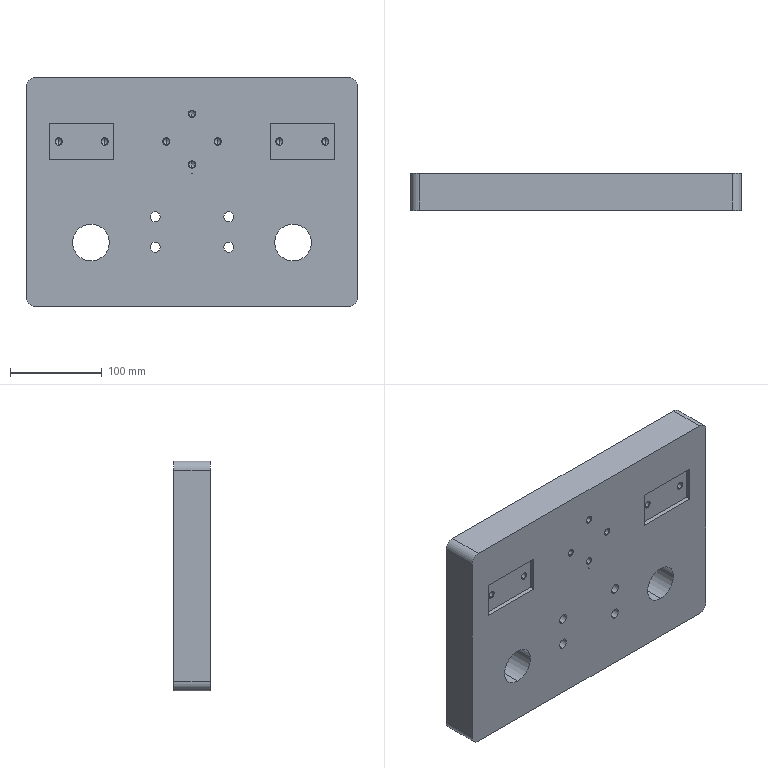Part | SolidWorks | features ICE 4, HoleWzd 3, Extrusion 1, MoveFace 1 | 1 solid | 101 faces | box 360 x 40 x 250 mm | volume 3399015 mm3 | cylinder 44 | cone 36 | plane 21 | commonest cylinder face diameters 6.8 x16 11 x8 18 x8 20 x4 40 x4 8.5 x2